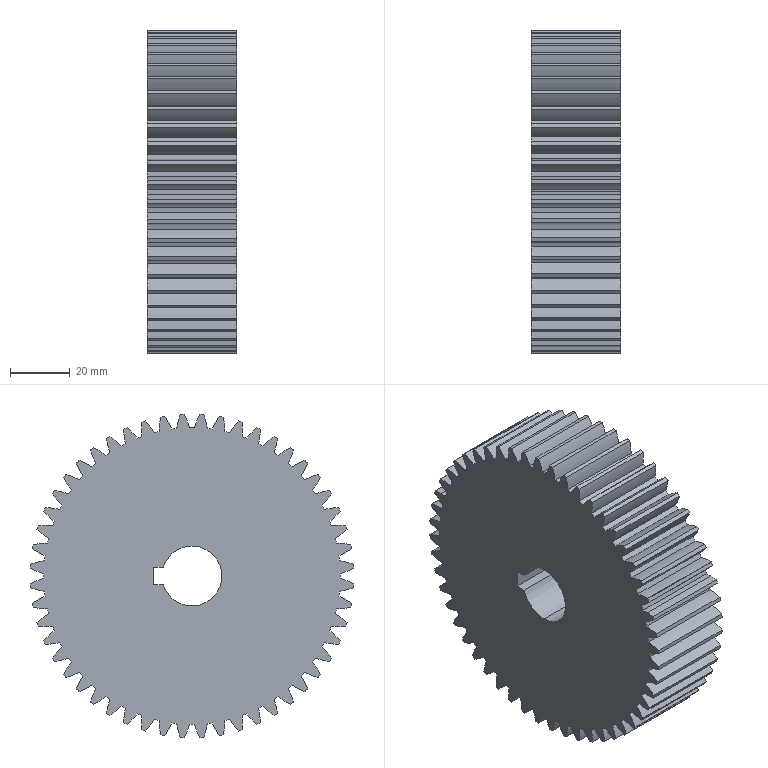Part | SolidWorks | features ICE 1, MBimport 1 | 1 solid | 221 faces | box 30 x 107.874 x 107.874 mm | volume 241879 mm3 | cylinder 216 | plane 5 | commonest cylinder face diameters 41.6 x108 98.998 x53 108 x52 20 x3